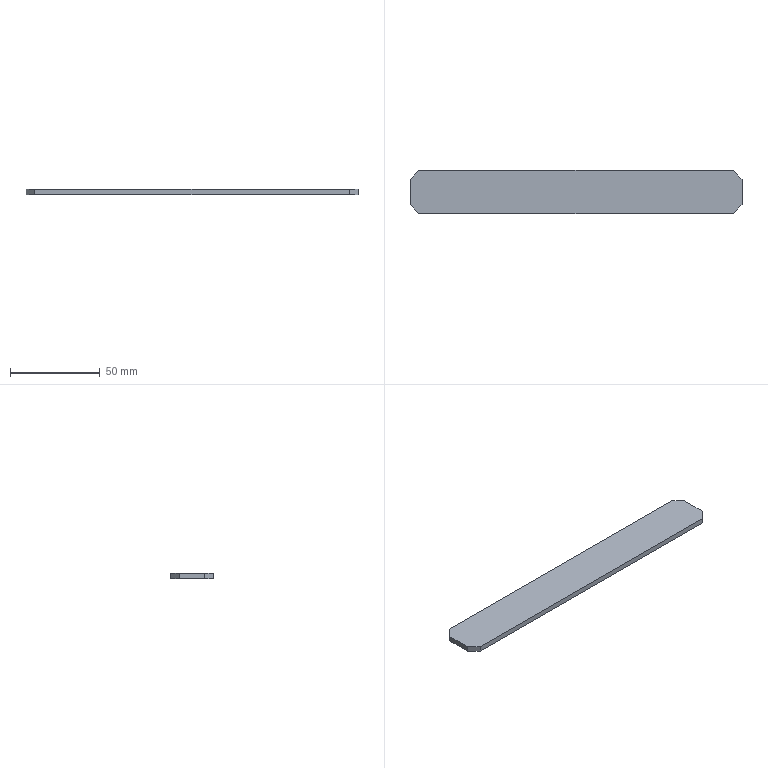Part | SolidWorks | features Extrusion 1 | 1 solid | 10 faces | box 185 x 24 x 3 mm | volume 13170 mm3 | plane 10
STEP:
#1=CARTESIAN_POINT('',(87.5,24.,0.));
#2=VERTEX_POINT('',#1);
#3=CARTESIAN_POINT('',(-87.5,24.,0.));
#4=VERTEX_POINT('',#3);
#5=CARTESIAN_POINT('',(-87.5,24.,0.));
#6=DIRECTION('',(-1.,0.,0.));
#7=VECTOR('',#6,1000.);
#8=LINE('',#5,#7);
#9=EDGE_CURVE('',#2,#4,#8,.T.);
#10=ORIENTED_EDGE('',*,*,#9,.T.);
#11=CARTESIAN_POINT('',(-87.5,24.,3.));
#12=VERTEX_POINT('',#11);
#13=CARTESIAN_POINT('',(-87.5,24.,3.));
#14=DIRECTION('',(0.,0.,-1.));
#15=VECTOR('',#14,1000.);
#16=LINE('',#13,#15);
#17=EDGE_CURVE('',#12,#4,#16,.T.);
#18=ORIENTED_EDGE('',*,*,#17,.F.);
#19=CARTESIAN_POINT('',(87.5,24.,3.));
#20=VERTEX_POINT('',#19);
#21=CARTESIAN_POINT('',(-87.5,24.,3.));
#22=DIRECTION('',(-1.,0.,0.));
#23=VECTOR('',#22,1000.);
#24=LINE('',#21,#23);
#25=EDGE_CURVE('',#20,#12,#24,.T.);
#26=ORIENTED_EDGE('',*,*,#25,.F.);
#27=CARTESIAN_POINT('',(87.5,24.,3.));
#28=DIRECTION('',(0.,0.,-1.));
#29=VECTOR('',#28,1000.);
#30=LINE('',#27,#29);
#31=EDGE_CURVE('',#20,#2,#30,.T.);
#32=ORIENTED_EDGE('',*,*,#31,.T.);
#33=EDGE_LOOP('',(#10,#18,#26,#32));
#34=FACE_OUTER_BOUND('',#33,.T.);
#35=CARTESIAN_POINT('',(-87.5,24.,3.));
#36=DIRECTION('',(0.,-1.,0.));
#37=DIRECTION('',(0.,0.,-1.));
#38=AXIS2_PLACEMENT_3D('',#35,#36,#37);
#39=PLANE('',#38);
#40=ADVANCED_FACE('',(#34),#39,.F.);
#41=CARTESIAN_POINT('',(-92.5,19.,0.));
#42=VERTEX_POINT('',#41);
#43=CARTESIAN_POINT('',(-92.5,19.,0.));
#44=DIRECTION('',(-0.7071,-0.7071,0.));
#45=VECTOR('',#44,1000.);
#46=LINE('',#43,#45);
#47=EDGE_CURVE('',#4,#42,#46,.T.);
#48=ORIENTED_EDGE('',*,*,#47,.T.);
#49=CARTESIAN_POINT('',(-92.5,19.,3.));
#50=VERTEX_POINT('',#49);
#51=CARTESIAN_POINT('',(-92.5,19.,3.));
#52=DIRECTION('',(0.,0.,-1.));
#53=VECTOR('',#52,1000.);
#54=LINE('',#51,#53);
#55=EDGE_CURVE('',#50,#42,#54,.T.);
#56=ORIENTED_EDGE('',*,*,#55,.F.);
#57=CARTESIAN_POINT('',(-92.5,19.,3.));
#58=DIRECTION('',(-0.7071,-0.7071,0.));
#59=VECTOR('',#58,1000.);
#60=LINE('',#57,#59);
#61=EDGE_CURVE('',#12,#50,#60,.T.);
#62=ORIENTED_EDGE('',*,*,#61,.F.);
#63=ORIENTED_EDGE('',*,*,#17,.T.);
#64=EDGE_LOOP('',(#48,#56,#62,#63));
#65=FACE_OUTER_BOUND('',#64,.T.);
#66=CARTESIAN_POINT('',(-92.5,19.,3.));
#67=DIRECTION('',(0.7071,-0.7071,0.));
#68=DIRECTION('',(0.7071,0.7071,0.));
#69=AXIS2_PLACEMENT_3D('',#66,#67,#68);
#70=PLANE('',#69);
#71=ADVANCED_FACE('',(#65),#70,.F.);
#72=CARTESIAN_POINT('',(-92.5,5.,0.));
#73=VERTEX_POINT('',#72);
#74=CARTESIAN_POINT('',(-92.5,19.,0.));
#75=DIRECTION('',(0.,-1.,0.));
#76=VECTOR('',#75,1000.);
#77=LINE('',#74,#76);
#78=EDGE_CURVE('',#42,#73,#77,.T.);
#79=ORIENTED_EDGE('',*,*,#78,.T.);
#80=CARTESIAN_POINT('',(-92.5,5.,3.));
#81=VERTEX_POINT('',#80);
#82=CARTESIAN_POINT('',(-92.5,5.,3.));
#83=DIRECTION('',(0.,0.,-1.));
#84=VECTOR('',#83,1000.);
#85=LINE('',#82,#84);
#86=EDGE_CURVE('',#81,#73,#85,.T.);
#87=ORIENTED_EDGE('',*,*,#86,.F.);
#88=CARTESIAN_POINT('',(-92.5,19.,3.));
#89=DIRECTION('',(0.,-1.,0.));
#90=VECTOR('',#89,1000.);
#91=LINE('',#88,#90);
#92=EDGE_CURVE('',#50,#81,#91,.T.);
#93=ORIENTED_EDGE('',*,*,#92,.F.);
#94=ORIENTED_EDGE('',*,*,#55,.T.);
#95=EDGE_LOOP('',(#79,#87,#93,#94));
#96=FACE_OUTER_BOUND('',#95,.T.);
#97=CARTESIAN_POINT('',(-92.5,19.,3.));
#98=DIRECTION('',(1.,0.,0.));
#99=DIRECTION('',(0.,0.,-1.));
#100=AXIS2_PLACEMENT_3D('',#97,#98,#99);
#101=PLANE('',#100);
#102=ADVANCED_FACE('',(#96),#101,.F.);
#103=CARTESIAN_POINT('',(-87.5,0.,0.));
#104=VERTEX_POINT('',#103);
#105=CARTESIAN_POINT('',(-92.5,5.,0.));
#106=DIRECTION('',(0.7071,-0.7071,0.));
#107=VECTOR('',#106,1000.);
#108=LINE('',#105,#107);
#109=EDGE_CURVE('',#73,#104,#108,.T.);
#110=ORIENTED_EDGE('',*,*,#109,.T.);
#111=CARTESIAN_POINT('',(-87.5,0.,3.));
#112=VERTEX_POINT('',#111);
#113=CARTESIAN_POINT('',(-87.5,0.,3.));
#114=DIRECTION('',(0.,0.,-1.));
#115=VECTOR('',#114,1000.);
#116=LINE('',#113,#115);
#117=EDGE_CURVE('',#112,#104,#116,.T.);
#118=ORIENTED_EDGE('',*,*,#117,.F.);
#119=CARTESIAN_POINT('',(-92.5,5.,3.));
#120=DIRECTION('',(0.7071,-0.7071,0.));
#121=VECTOR('',#120,1000.);
#122=LINE('',#119,#121);
#123=EDGE_CURVE('',#81,#112,#122,.T.);
#124=ORIENTED_EDGE('',*,*,#123,.F.);
#125=ORIENTED_EDGE('',*,*,#86,.T.);
#126=EDGE_LOOP('',(#110,#118,#124,#125));
#127=FACE_OUTER_BOUND('',#126,.T.);
#128=CARTESIAN_POINT('',(-92.5,5.,3.));
#129=DIRECTION('',(0.7071,0.7071,0.));
#130=DIRECTION('',(-0.7071,0.7071,0.));
#131=AXIS2_PLACEMENT_3D('',#128,#129,#130);
#132=PLANE('',#131);
#133=ADVANCED_FACE('',(#127),#132,.F.);
#134=CARTESIAN_POINT('',(87.5,0.,0.));
#135=VERTEX_POINT('',#134);
#136=CARTESIAN_POINT('',(-87.5,0.,0.));
#137=DIRECTION('',(1.,0.,0.));
#138=VECTOR('',#137,1000.);
#139=LINE('',#136,#138);
#140=EDGE_CURVE('',#104,#135,#139,.T.);
#141=ORIENTED_EDGE('',*,*,#140,.T.);
#142=CARTESIAN_POINT('',(87.5,0.,3.));
#143=VERTEX_POINT('',#142);
#144=CARTESIAN_POINT('',(87.5,0.,3.));
#145=DIRECTION('',(0.,0.,-1.));
#146=VECTOR('',#145,1000.);
#147=LINE('',#144,#146);
#148=EDGE_CURVE('',#143,#135,#147,.T.);
#149=ORIENTED_EDGE('',*,*,#148,.F.);
#150=CARTESIAN_POINT('',(-87.5,0.,3.));
#151=DIRECTION('',(1.,0.,0.));
#152=VECTOR('',#151,1000.);
#153=LINE('',#150,#152);
#154=EDGE_CURVE('',#112,#143,#153,.T.);
#155=ORIENTED_EDGE('',*,*,#154,.F.);
#156=ORIENTED_EDGE('',*,*,#117,.T.);
#157=EDGE_LOOP('',(#141,#149,#155,#156));
#158=FACE_OUTER_BOUND('',#157,.T.);
#159=CARTESIAN_POINT('',(-87.5,0.,3.));
#160=DIRECTION('',(0.,1.,0.));
#161=DIRECTION('',(-1.,0.,0.));
#162=AXIS2_PLACEMENT_3D('',#159,#160,#161);
#163=PLANE('',#162);
#164=ADVANCED_FACE('',(#158),#163,.F.);
#165=CARTESIAN_POINT('',(92.5,5.,0.));
#166=VERTEX_POINT('',#165);
#167=CARTESIAN_POINT('',(87.5,0.,0.));
#168=DIRECTION('',(0.7071,0.7071,0.));
#169=VECTOR('',#168,1000.);
#170=LINE('',#167,#169);
#171=EDGE_CURVE('',#135,#166,#170,.T.);
#172=ORIENTED_EDGE('',*,*,#171,.T.);
#173=CARTESIAN_POINT('',(92.5,5.,3.));
#174=VERTEX_POINT('',#173);
#175=CARTESIAN_POINT('',(92.5,5.,3.));
#176=DIRECTION('',(0.,0.,-1.));
#177=VECTOR('',#176,1000.);
#178=LINE('',#175,#177);
#179=EDGE_CURVE('',#174,#166,#178,.T.);
#180=ORIENTED_EDGE('',*,*,#179,.F.);
#181=CARTESIAN_POINT('',(87.5,0.,3.));
#182=DIRECTION('',(0.7071,0.7071,0.));
#183=VECTOR('',#182,1000.);
#184=LINE('',#181,#183);
#185=EDGE_CURVE('',#143,#174,#184,.T.);
#186=ORIENTED_EDGE('',*,*,#185,.F.);
#187=ORIENTED_EDGE('',*,*,#148,.T.);
#188=EDGE_LOOP('',(#172,#180,#186,#187));
#189=FACE_OUTER_BOUND('',#188,.T.);
#190=CARTESIAN_POINT('',(87.5,0.,3.));
#191=DIRECTION('',(-0.7071,0.7071,0.));
#192=DIRECTION('',(-0.7071,-0.7071,0.));
#193=AXIS2_PLACEMENT_3D('',#190,#191,#192);
#194=PLANE('',#193);
#195=ADVANCED_FACE('',(#189),#194,.F.);
#196=CARTESIAN_POINT('',(92.5,19.,0.));
#197=VERTEX_POINT('',#196);
#198=CARTESIAN_POINT('',(92.5,19.,0.));
#199=DIRECTION('',(0.,1.,0.));
#200=VECTOR('',#199,1000.);
#201=LINE('',#198,#200);
#202=EDGE_CURVE('',#166,#197,#201,.T.);
#203=ORIENTED_EDGE('',*,*,#202,.T.);
#204=CARTESIAN_POINT('',(92.5,19.,3.));
#205=VERTEX_POINT('',#204);
#206=CARTESIAN_POINT('',(92.5,19.,3.));
#207=DIRECTION('',(0.,0.,-1.));
#208=VECTOR('',#207,1000.);
#209=LINE('',#206,#208);
#210=EDGE_CURVE('',#205,#197,#209,.T.);
#211=ORIENTED_EDGE('',*,*,#210,.F.);
#212=CARTESIAN_POINT('',(92.5,19.,3.));
#213=DIRECTION('',(0.,1.,0.));
#214=VECTOR('',#213,1000.);
#215=LINE('',#212,#214);
#216=EDGE_CURVE('',#174,#205,#215,.T.);
#217=ORIENTED_EDGE('',*,*,#216,.F.);
#218=ORIENTED_EDGE('',*,*,#179,.T.);
#219=EDGE_LOOP('',(#203,#211,#217,#218));
#220=FACE_OUTER_BOUND('',#219,.T.);
#221=CARTESIAN_POINT('',(92.5,19.,3.));
#222=DIRECTION('',(-1.,0.,0.));
#223=DIRECTION('',(0.,0.,1.));
#224=AXIS2_PLACEMENT_3D('',#221,#222,#223);
#225=PLANE('',#224);
#226=ADVANCED_FACE('',(#220),#225,.F.);
#227=CARTESIAN_POINT('',(87.5,24.,0.));
#228=DIRECTION('',(-0.7071,0.7071,0.));
#229=VECTOR('',#228,1000.);
#230=LINE('',#227,#229);
#231=EDGE_CURVE('',#197,#2,#230,.T.);
#232=ORIENTED_EDGE('',*,*,#231,.T.);
#233=ORIENTED_EDGE('',*,*,#31,.F.);
#234=CARTESIAN_POINT('',(87.5,24.,3.));
#235=DIRECTION('',(-0.7071,0.7071,0.));
#236=VECTOR('',#235,1000.);
#237=LINE('',#234,#236);
#238=EDGE_CURVE('',#205,#20,#237,.T.);
#239=ORIENTED_EDGE('',*,*,#238,.F.);
#240=ORIENTED_EDGE('',*,*,#210,.T.);
#241=EDGE_LOOP('',(#232,#233,#239,#240));
#242=FACE_OUTER_BOUND('',#241,.T.);
#243=CARTESIAN_POINT('',(87.5,24.,3.));
#244=DIRECTION('',(-0.7071,-0.7071,0.));
#245=DIRECTION('',(0.7071,-0.7071,0.));
#246=AXIS2_PLACEMENT_3D('',#243,#244,#245);
#247=PLANE('',#246);
#248=ADVANCED_FACE('',(#242),#247,.F.);
#249=ORIENTED_EDGE('',*,*,#25,.T.);
#250=ORIENTED_EDGE('',*,*,#61,.T.);
#251=ORIENTED_EDGE('',*,*,#92,.T.);
#252=ORIENTED_EDGE('',*,*,#123,.T.);
#253=ORIENTED_EDGE('',*,*,#154,.T.);
#254=ORIENTED_EDGE('',*,*,#185,.T.);
#255=ORIENTED_EDGE('',*,*,#216,.T.);
#256=ORIENTED_EDGE('',*,*,#238,.T.);
#257=EDGE_LOOP('',(#249,#250,#251,#252,#253,#254,#255,#256));
#258=FACE_OUTER_BOUND('',#257,.T.);
#259=CARTESIAN_POINT('',(0.,0.,3.));
#260=DIRECTION('',(0.,0.,-1.));
#261=DIRECTION('',(-1.,0.,0.));
#262=AXIS2_PLACEMENT_3D('',#259,#260,#261);
#263=PLANE('',#262);
#264=ADVANCED_FACE('',(#258),#263,.F.);
#265=ORIENTED_EDGE('',*,*,#9,.F.);
#266=ORIENTED_EDGE('',*,*,#231,.F.);
#267=ORIENTED_EDGE('',*,*,#202,.F.);
#268=ORIENTED_EDGE('',*,*,#171,.F.);
#269=ORIENTED_EDGE('',*,*,#140,.F.);
#270=ORIENTED_EDGE('',*,*,#109,.F.);
#271=ORIENTED_EDGE('',*,*,#78,.F.);
#272=ORIENTED_EDGE('',*,*,#47,.F.);
#273=EDGE_LOOP('',(#265,#266,#267,#268,#269,#270,#271,#272));
#274=FACE_OUTER_BOUND('',#273,.T.);
#275=CARTESIAN_POINT('',(0.,0.,0.));
#276=DIRECTION('',(0.,0.,-1.));
#277=DIRECTION('',(-1.,0.,0.));
#278=AXIS2_PLACEMENT_3D('',#275,#276,#277);
#279=PLANE('',#278);
#280=ADVANCED_FACE('',(#274),#279,.T.);
#281=CLOSED_SHELL('',(#40,#71,#102,#133,#164,#195,#226,#248,#264,#280));
#282=MANIFOLD_SOLID_BREP('',#281);
#283=CARTESIAN_POINT('',(0.,0.,0.));
#284=DIRECTION('',(0.,0.,1.));
#285=DIRECTION('',(1.,0.,0.));
#286=AXIS2_PLACEMENT_3D('',#283,#284,#285);
#287=(LENGTH_UNIT()NAMED_UNIT(*)SI_UNIT(.MILLI.,.METRE.));
#288=UNCERTAINTY_MEASURE_WITH_UNIT(LENGTH_MEASURE(0.00001),#287,'','');
#289=(NAMED_UNIT(*)PLANE_ANGLE_UNIT()SI_UNIT($,.RADIAN.));
#290=(NAMED_UNIT(*)SI_UNIT($,.STERADIAN.)SOLID_ANGLE_UNIT());
#291=(GEOMETRIC_REPRESENTATION_CONTEXT(3)GLOBAL_UNCERTAINTY_ASSIGNED_CONTEXT((#288))GLOBAL_UNIT_ASSIGNED_CONTEXT((#287,#289,#290))REPRESENTATION_CONTEXT('',''));
#292=ADVANCED_BREP_SHAPE_REPRESENTATION('',(#282,#286),#291);